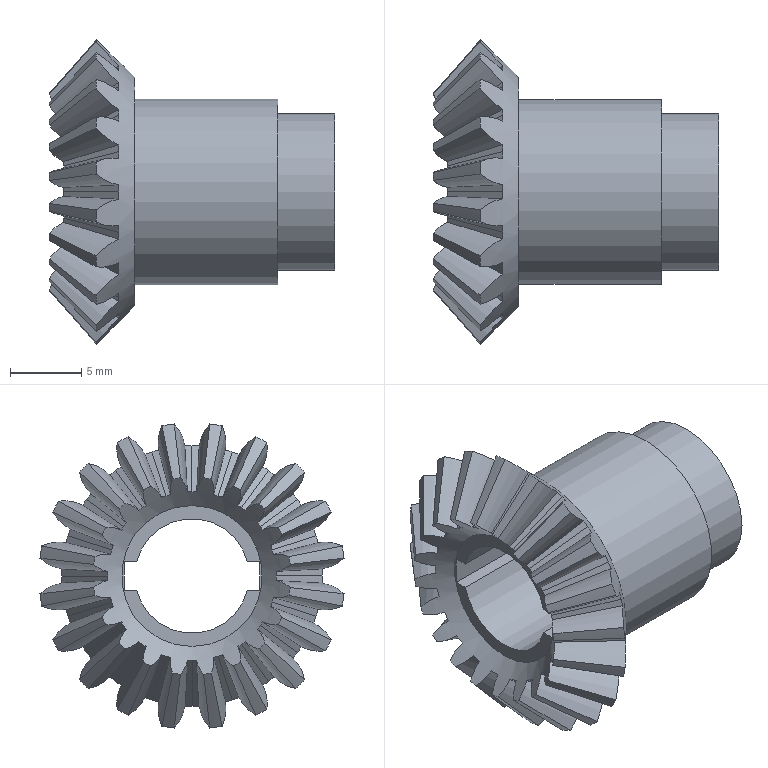Part | NX | features EXTRACT_BODY 20, TRIM BODY 20, Instance Feature 19, DATUM_CSYS 3, SKETCH 2, EXTEND_SHEET 1, EXTRUDE 1, Pattern Feature 1, SKIN 1, SWP104 1 | 1 solid | 116 faces | box 19.993 x 21.268 x 21.268 mm | volume 1845 mm3 | plane 50 | spline 40 | cone 22 | cylinder 4 | commonest cylinder face diameters 8 x2 11 x1 13 x1